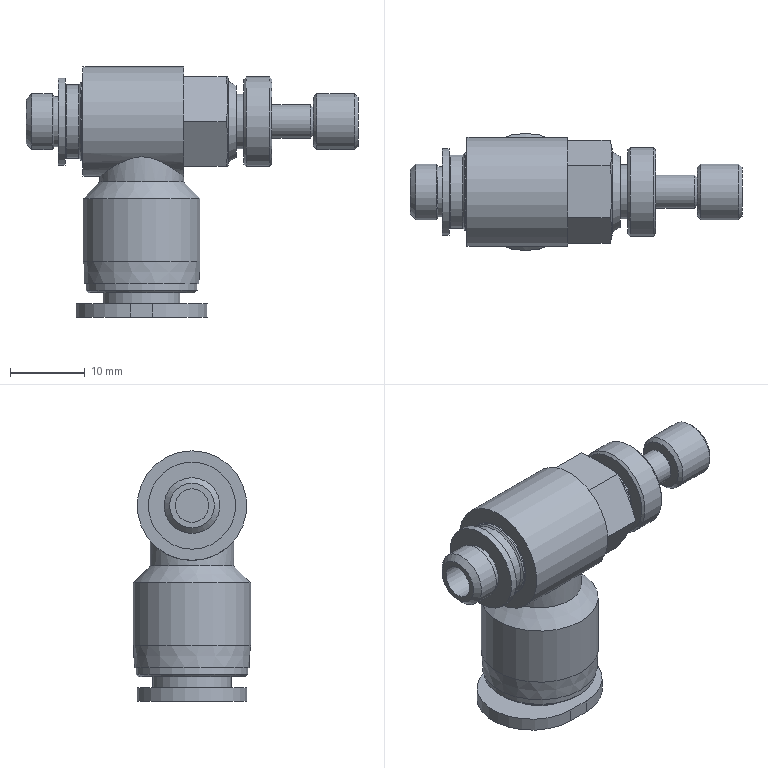Part | NX | features J-XZB01-D6-M5.SLDPRT 2 | 1 solid | 58 faces | box 44.567 x 15.75 x 33.6 mm | volume 6449 mm3 | plane 25 | cylinder 18 | cone 14 | torus 1 | commonest cylinder face diameters 14.7 x3 4.5 x2 7.5 x2 10.5 x2 6.75 x1 7.35 x1